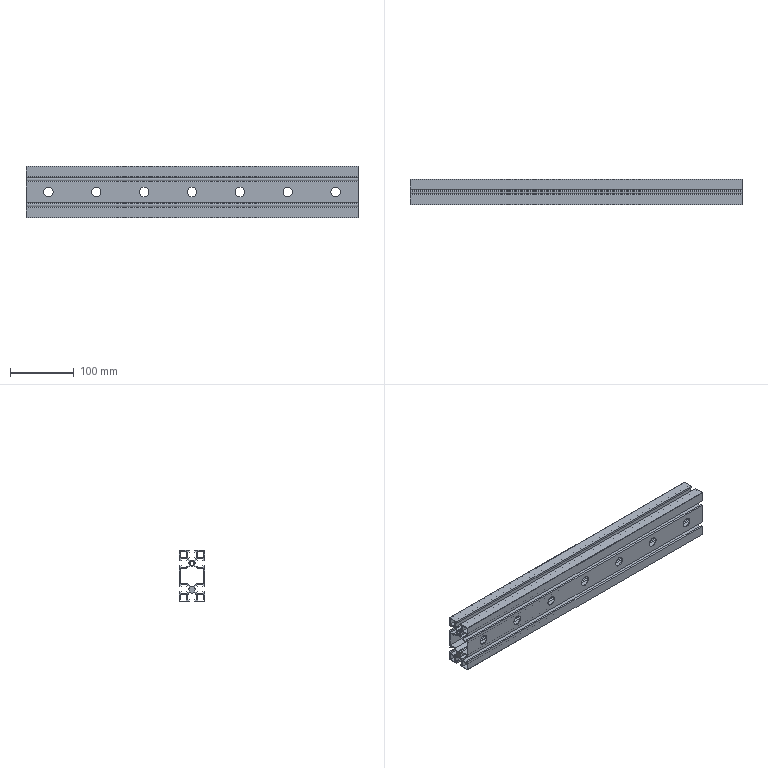Part | STEP file | 1 solid | 152 faces | box 520 x 40 x 80 mm | volume 382140 mm3 | plane 110 | cylinder 42 | commonest cylinder face diameters 15 x28 9.6 x9 0.6 x2 6.6 x2 13.3 x1